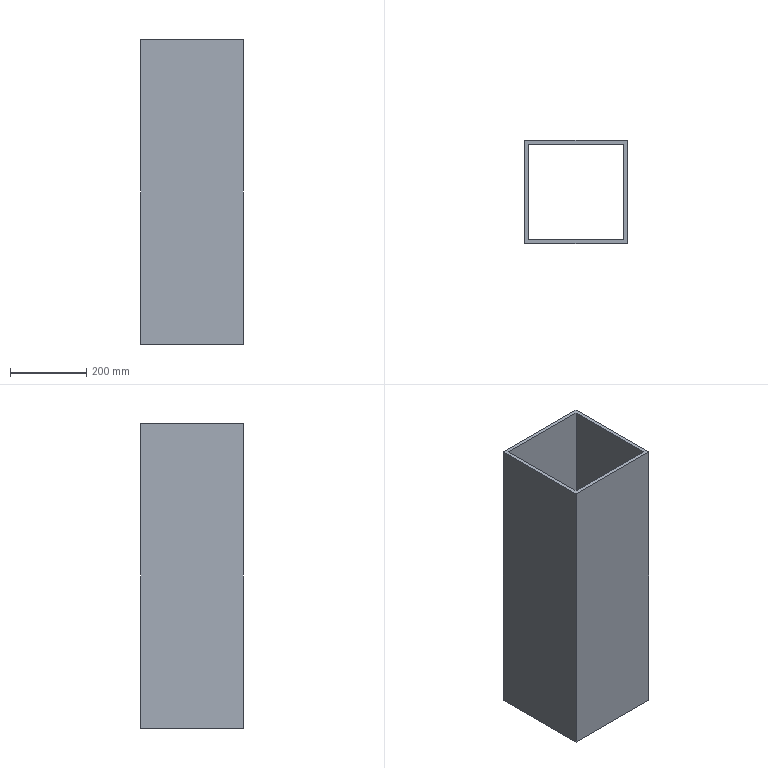Part | SolidWorks | features ExtruThin 1 | 1 solid | 10 faces | box 270 x 270 x 800 mm | volume 8320000 mm3 | plane 10
STEP:
#1=CARTESIAN_POINT('',(-135.,135.,800.));
#2=VERTEX_POINT('',#1);
#3=CARTESIAN_POINT('',(-135.,-135.,800.));
#4=VERTEX_POINT('',#3);
#5=CARTESIAN_POINT('',(-135.,0.,800.));
#6=DIRECTION('',(0.,-1.,0.));
#7=VECTOR('',#6,1000.);
#8=LINE('',#5,#7);
#9=EDGE_CURVE('',#2,#4,#8,.T.);
#10=ORIENTED_EDGE('',*,*,#9,.T.);
#11=CARTESIAN_POINT('',(135.,-135.,800.));
#12=VERTEX_POINT('',#11);
#13=CARTESIAN_POINT('',(0.,-135.,800.));
#14=DIRECTION('',(1.,0.,0.));
#15=VECTOR('',#14,1000.);
#16=LINE('',#13,#15);
#17=EDGE_CURVE('',#4,#12,#16,.T.);
#18=ORIENTED_EDGE('',*,*,#17,.T.);
#19=CARTESIAN_POINT('',(135.,135.,800.));
#20=VERTEX_POINT('',#19);
#21=CARTESIAN_POINT('',(135.,0.,800.));
#22=DIRECTION('',(0.,1.,0.));
#23=VECTOR('',#22,1000.);
#24=LINE('',#21,#23);
#25=EDGE_CURVE('',#12,#20,#24,.T.);
#26=ORIENTED_EDGE('',*,*,#25,.T.);
#27=CARTESIAN_POINT('',(0.,135.,800.));
#28=DIRECTION('',(-1.,0.,0.));
#29=VECTOR('',#28,1000.);
#30=LINE('',#27,#29);
#31=EDGE_CURVE('',#20,#2,#30,.T.);
#32=ORIENTED_EDGE('',*,*,#31,.T.);
#33=EDGE_LOOP('',(#10,#18,#26,#32));
#34=FACE_OUTER_BOUND('',#33,.T.);
#35=CARTESIAN_POINT('',(-125.,-125.,800.));
#36=VERTEX_POINT('',#35);
#37=CARTESIAN_POINT('',(125.,-125.,800.));
#38=VERTEX_POINT('',#37);
#39=CARTESIAN_POINT('',(125.,-125.,800.));
#40=DIRECTION('',(1.,0.,0.));
#41=VECTOR('',#40,1000.);
#42=LINE('',#39,#41);
#43=EDGE_CURVE('',#36,#38,#42,.T.);
#44=ORIENTED_EDGE('',*,*,#43,.F.);
#45=CARTESIAN_POINT('',(-125.,125.,800.));
#46=VERTEX_POINT('',#45);
#47=CARTESIAN_POINT('',(-125.,125.,800.));
#48=DIRECTION('',(0.,-1.,0.));
#49=VECTOR('',#48,1000.);
#50=LINE('',#47,#49);
#51=EDGE_CURVE('',#46,#36,#50,.T.);
#52=ORIENTED_EDGE('',*,*,#51,.F.);
#53=CARTESIAN_POINT('',(125.,125.,800.));
#54=VERTEX_POINT('',#53);
#55=CARTESIAN_POINT('',(125.,125.,800.));
#56=DIRECTION('',(-1.,0.,0.));
#57=VECTOR('',#56,1000.);
#58=LINE('',#55,#57);
#59=EDGE_CURVE('',#54,#46,#58,.T.);
#60=ORIENTED_EDGE('',*,*,#59,.F.);
#61=CARTESIAN_POINT('',(125.,125.,800.));
#62=DIRECTION('',(0.,1.,0.));
#63=VECTOR('',#62,1000.);
#64=LINE('',#61,#63);
#65=EDGE_CURVE('',#38,#54,#64,.T.);
#66=ORIENTED_EDGE('',*,*,#65,.F.);
#67=EDGE_LOOP('',(#44,#52,#60,#66));
#68=FACE_BOUND('',#67,.T.);
#69=CARTESIAN_POINT('',(0.,0.,800.));
#70=DIRECTION('',(0.,0.,1.));
#71=DIRECTION('',(1.,0.,0.));
#72=AXIS2_PLACEMENT_3D('',#69,#70,#71);
#73=PLANE('',#72);
#74=ADVANCED_FACE('',(#34,#68),#73,.T.);
#75=CARTESIAN_POINT('',(-135.,135.,0.));
#76=VERTEX_POINT('',#75);
#77=CARTESIAN_POINT('',(-135.,-135.,0.));
#78=VERTEX_POINT('',#77);
#79=CARTESIAN_POINT('',(-135.,0.,0.));
#80=DIRECTION('',(0.,-1.,0.));
#81=VECTOR('',#80,1000.);
#82=LINE('',#79,#81);
#83=EDGE_CURVE('',#76,#78,#82,.T.);
#84=ORIENTED_EDGE('',*,*,#83,.F.);
#85=CARTESIAN_POINT('',(135.,135.,0.));
#86=VERTEX_POINT('',#85);
#87=CARTESIAN_POINT('',(0.,135.,0.));
#88=DIRECTION('',(-1.,0.,0.));
#89=VECTOR('',#88,1000.);
#90=LINE('',#87,#89);
#91=EDGE_CURVE('',#86,#76,#90,.T.);
#92=ORIENTED_EDGE('',*,*,#91,.F.);
#93=CARTESIAN_POINT('',(135.,-135.,0.));
#94=VERTEX_POINT('',#93);
#95=CARTESIAN_POINT('',(135.,0.,0.));
#96=DIRECTION('',(0.,1.,0.));
#97=VECTOR('',#96,1000.);
#98=LINE('',#95,#97);
#99=EDGE_CURVE('',#94,#86,#98,.T.);
#100=ORIENTED_EDGE('',*,*,#99,.F.);
#101=CARTESIAN_POINT('',(0.,-135.,0.));
#102=DIRECTION('',(1.,0.,0.));
#103=VECTOR('',#102,1000.);
#104=LINE('',#101,#103);
#105=EDGE_CURVE('',#78,#94,#104,.T.);
#106=ORIENTED_EDGE('',*,*,#105,.F.);
#107=EDGE_LOOP('',(#84,#92,#100,#106));
#108=FACE_OUTER_BOUND('',#107,.T.);
#109=CARTESIAN_POINT('',(-125.,125.,0.));
#110=VERTEX_POINT('',#109);
#111=CARTESIAN_POINT('',(-125.,-125.,0.));
#112=VERTEX_POINT('',#111);
#113=CARTESIAN_POINT('',(-125.,125.,0.));
#114=DIRECTION('',(0.,-1.,0.));
#115=VECTOR('',#114,1000.);
#116=LINE('',#113,#115);
#117=EDGE_CURVE('',#110,#112,#116,.T.);
#118=ORIENTED_EDGE('',*,*,#117,.T.);
#119=CARTESIAN_POINT('',(125.,-125.,0.));
#120=VERTEX_POINT('',#119);
#121=CARTESIAN_POINT('',(125.,-125.,0.));
#122=DIRECTION('',(1.,0.,0.));
#123=VECTOR('',#122,1000.);
#124=LINE('',#121,#123);
#125=EDGE_CURVE('',#112,#120,#124,.T.);
#126=ORIENTED_EDGE('',*,*,#125,.T.);
#127=CARTESIAN_POINT('',(125.,125.,0.));
#128=VERTEX_POINT('',#127);
#129=CARTESIAN_POINT('',(125.,125.,0.));
#130=DIRECTION('',(0.,1.,0.));
#131=VECTOR('',#130,1000.);
#132=LINE('',#129,#131);
#133=EDGE_CURVE('',#120,#128,#132,.T.);
#134=ORIENTED_EDGE('',*,*,#133,.T.);
#135=CARTESIAN_POINT('',(125.,125.,0.));
#136=DIRECTION('',(-1.,0.,0.));
#137=VECTOR('',#136,1000.);
#138=LINE('',#135,#137);
#139=EDGE_CURVE('',#128,#110,#138,.T.);
#140=ORIENTED_EDGE('',*,*,#139,.T.);
#141=EDGE_LOOP('',(#118,#126,#134,#140));
#142=FACE_BOUND('',#141,.T.);
#143=CARTESIAN_POINT('',(0.,0.,0.));
#144=DIRECTION('',(0.,0.,1.));
#145=DIRECTION('',(1.,0.,0.));
#146=AXIS2_PLACEMENT_3D('',#143,#144,#145);
#147=PLANE('',#146);
#148=ADVANCED_FACE('',(#108,#142),#147,.F.);
#149=ORIENTED_EDGE('',*,*,#83,.T.);
#150=CARTESIAN_POINT('',(-135.,-135.,800.));
#151=DIRECTION('',(0.,0.,-1.));
#152=VECTOR('',#151,1000.);
#153=LINE('',#150,#152);
#154=EDGE_CURVE('',#4,#78,#153,.T.);
#155=ORIENTED_EDGE('',*,*,#154,.F.);
#156=ORIENTED_EDGE('',*,*,#9,.F.);
#157=CARTESIAN_POINT('',(-135.,135.,800.));
#158=DIRECTION('',(0.,0.,-1.));
#159=VECTOR('',#158,1000.);
#160=LINE('',#157,#159);
#161=EDGE_CURVE('',#2,#76,#160,.T.);
#162=ORIENTED_EDGE('',*,*,#161,.T.);
#163=EDGE_LOOP('',(#149,#155,#156,#162));
#164=FACE_OUTER_BOUND('',#163,.T.);
#165=CARTESIAN_POINT('',(-135.,0.,800.));
#166=DIRECTION('',(1.,0.,0.));
#167=DIRECTION('',(0.,1.,0.));
#168=AXIS2_PLACEMENT_3D('',#165,#166,#167);
#169=PLANE('',#168);
#170=ADVANCED_FACE('',(#164),#169,.F.);
#171=ORIENTED_EDGE('',*,*,#105,.T.);
#172=CARTESIAN_POINT('',(135.,-135.,800.));
#173=DIRECTION('',(0.,0.,-1.));
#174=VECTOR('',#173,1000.);
#175=LINE('',#172,#174);
#176=EDGE_CURVE('',#12,#94,#175,.T.);
#177=ORIENTED_EDGE('',*,*,#176,.F.);
#178=ORIENTED_EDGE('',*,*,#17,.F.);
#179=ORIENTED_EDGE('',*,*,#154,.T.);
#180=EDGE_LOOP('',(#171,#177,#178,#179));
#181=FACE_OUTER_BOUND('',#180,.T.);
#182=CARTESIAN_POINT('',(0.,-135.,800.));
#183=DIRECTION('',(0.,1.,0.));
#184=DIRECTION('',(-1.,0.,0.));
#185=AXIS2_PLACEMENT_3D('',#182,#183,#184);
#186=PLANE('',#185);
#187=ADVANCED_FACE('',(#181),#186,.F.);
#188=ORIENTED_EDGE('',*,*,#99,.T.);
#189=CARTESIAN_POINT('',(135.,135.,800.));
#190=DIRECTION('',(0.,0.,-1.));
#191=VECTOR('',#190,1000.);
#192=LINE('',#189,#191);
#193=EDGE_CURVE('',#20,#86,#192,.T.);
#194=ORIENTED_EDGE('',*,*,#193,.F.);
#195=ORIENTED_EDGE('',*,*,#25,.F.);
#196=ORIENTED_EDGE('',*,*,#176,.T.);
#197=EDGE_LOOP('',(#188,#194,#195,#196));
#198=FACE_OUTER_BOUND('',#197,.T.);
#199=CARTESIAN_POINT('',(135.,0.,800.));
#200=DIRECTION('',(-1.,0.,0.));
#201=DIRECTION('',(0.,-1.,0.));
#202=AXIS2_PLACEMENT_3D('',#199,#200,#201);
#203=PLANE('',#202);
#204=ADVANCED_FACE('',(#198),#203,.F.);
#205=ORIENTED_EDGE('',*,*,#91,.T.);
#206=ORIENTED_EDGE('',*,*,#161,.F.);
#207=ORIENTED_EDGE('',*,*,#31,.F.);
#208=ORIENTED_EDGE('',*,*,#193,.T.);
#209=EDGE_LOOP('',(#205,#206,#207,#208));
#210=FACE_OUTER_BOUND('',#209,.T.);
#211=CARTESIAN_POINT('',(0.,135.,800.));
#212=DIRECTION('',(0.,-1.,0.));
#213=DIRECTION('',(1.,0.,0.));
#214=AXIS2_PLACEMENT_3D('',#211,#212,#213);
#215=PLANE('',#214);
#216=ADVANCED_FACE('',(#210),#215,.F.);
#217=ORIENTED_EDGE('',*,*,#117,.F.);
#218=CARTESIAN_POINT('',(-125.,125.,800.));
#219=DIRECTION('',(0.,0.,-1.));
#220=VECTOR('',#219,1000.);
#221=LINE('',#218,#220);
#222=EDGE_CURVE('',#46,#110,#221,.T.);
#223=ORIENTED_EDGE('',*,*,#222,.F.);
#224=ORIENTED_EDGE('',*,*,#51,.T.);
#225=CARTESIAN_POINT('',(-125.,-125.,800.));
#226=DIRECTION('',(0.,0.,-1.));
#227=VECTOR('',#226,1000.);
#228=LINE('',#225,#227);
#229=EDGE_CURVE('',#36,#112,#228,.T.);
#230=ORIENTED_EDGE('',*,*,#229,.T.);
#231=EDGE_LOOP('',(#217,#223,#224,#230));
#232=FACE_OUTER_BOUND('',#231,.T.);
#233=CARTESIAN_POINT('',(-125.,125.,800.));
#234=DIRECTION('',(1.,0.,0.));
#235=DIRECTION('',(0.,1.,0.));
#236=AXIS2_PLACEMENT_3D('',#233,#234,#235);
#237=PLANE('',#236);
#238=ADVANCED_FACE('',(#232),#237,.T.);
#239=ORIENTED_EDGE('',*,*,#125,.F.);
#240=ORIENTED_EDGE('',*,*,#229,.F.);
#241=ORIENTED_EDGE('',*,*,#43,.T.);
#242=CARTESIAN_POINT('',(125.,-125.,800.));
#243=DIRECTION('',(0.,0.,-1.));
#244=VECTOR('',#243,1000.);
#245=LINE('',#242,#244);
#246=EDGE_CURVE('',#38,#120,#245,.T.);
#247=ORIENTED_EDGE('',*,*,#246,.T.);
#248=EDGE_LOOP('',(#239,#240,#241,#247));
#249=FACE_OUTER_BOUND('',#248,.T.);
#250=CARTESIAN_POINT('',(125.,-125.,800.));
#251=DIRECTION('',(0.,1.,0.));
#252=DIRECTION('',(-1.,0.,0.));
#253=AXIS2_PLACEMENT_3D('',#250,#251,#252);
#254=PLANE('',#253);
#255=ADVANCED_FACE('',(#249),#254,.T.);
#256=ORIENTED_EDGE('',*,*,#133,.F.);
#257=ORIENTED_EDGE('',*,*,#246,.F.);
#258=ORIENTED_EDGE('',*,*,#65,.T.);
#259=CARTESIAN_POINT('',(125.,125.,800.));
#260=DIRECTION('',(0.,0.,-1.));
#261=VECTOR('',#260,1000.);
#262=LINE('',#259,#261);
#263=EDGE_CURVE('',#54,#128,#262,.T.);
#264=ORIENTED_EDGE('',*,*,#263,.T.);
#265=EDGE_LOOP('',(#256,#257,#258,#264));
#266=FACE_OUTER_BOUND('',#265,.T.);
#267=CARTESIAN_POINT('',(125.,125.,800.));
#268=DIRECTION('',(-1.,0.,0.));
#269=DIRECTION('',(0.,-1.,0.));
#270=AXIS2_PLACEMENT_3D('',#267,#268,#269);
#271=PLANE('',#270);
#272=ADVANCED_FACE('',(#266),#271,.T.);
#273=ORIENTED_EDGE('',*,*,#139,.F.);
#274=ORIENTED_EDGE('',*,*,#263,.F.);
#275=ORIENTED_EDGE('',*,*,#59,.T.);
#276=ORIENTED_EDGE('',*,*,#222,.T.);
#277=EDGE_LOOP('',(#273,#274,#275,#276));
#278=FACE_OUTER_BOUND('',#277,.T.);
#279=CARTESIAN_POINT('',(125.,125.,800.));
#280=DIRECTION('',(0.,-1.,0.));
#281=DIRECTION('',(1.,0.,0.));
#282=AXIS2_PLACEMENT_3D('',#279,#280,#281);
#283=PLANE('',#282);
#284=ADVANCED_FACE('',(#278),#283,.T.);
#285=CLOSED_SHELL('',(#74,#148,#170,#187,#204,#216,#238,#255,#272,#284));
#286=MANIFOLD_SOLID_BREP('',#285);
#287=CARTESIAN_POINT('',(0.,0.,0.));
#288=DIRECTION('',(0.,0.,1.));
#289=DIRECTION('',(1.,0.,0.));
#290=AXIS2_PLACEMENT_3D('',#287,#288,#289);
#291=(LENGTH_UNIT()NAMED_UNIT(*)SI_UNIT(.MILLI.,.METRE.));
#292=UNCERTAINTY_MEASURE_WITH_UNIT(LENGTH_MEASURE(0.00001),#291,'','');
#293=(NAMED_UNIT(*)PLANE_ANGLE_UNIT()SI_UNIT($,.RADIAN.));
#294=(NAMED_UNIT(*)SI_UNIT($,.STERADIAN.)SOLID_ANGLE_UNIT());
#295=(GEOMETRIC_REPRESENTATION_CONTEXT(3)GLOBAL_UNCERTAINTY_ASSIGNED_CONTEXT((#292))GLOBAL_UNIT_ASSIGNED_CONTEXT((#291,#293,#294))REPRESENTATION_CONTEXT('',''));
#296=ADVANCED_BREP_SHAPE_REPRESENTATION('',(#286,#290),#295);